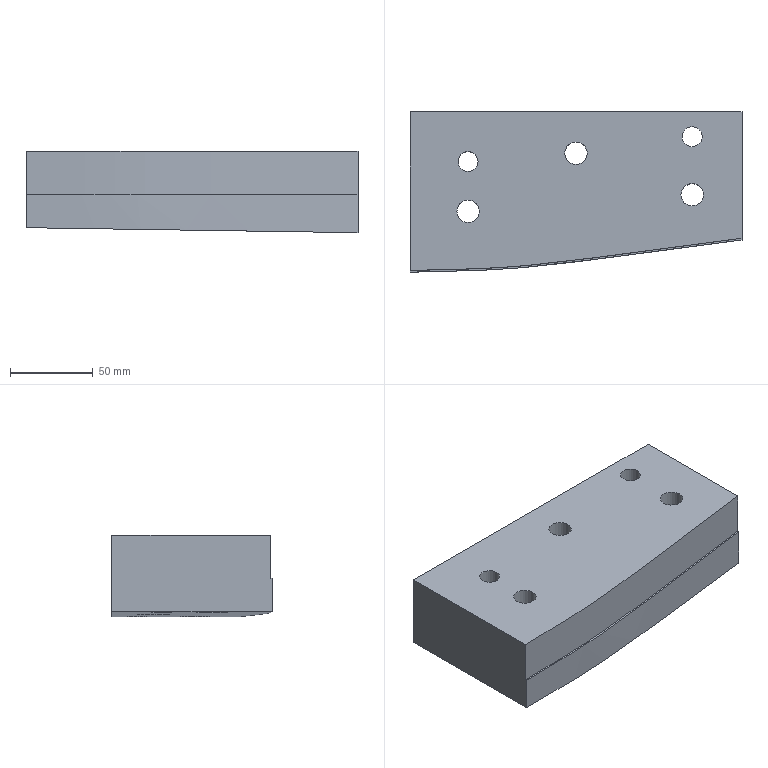Part | NX | features solid 2 | 1 solid | 23 faces | box 200 x 96.579 x 49 mm | volume 800737 mm3 | plane 11 | cylinder 10 | spline 2 | commonest cylinder face diameters 13.5 x3 19.5 x3 12 x2 13 x2
STEP:
#1=CARTESIAN_POINT('',(130.,110.798,14.));
#2=VERTEX_POINT('',#1);
#3=CARTESIAN_POINT('',(130.,111.807,14.));
#4=VERTEX_POINT('',#3);
#5=CARTESIAN_POINT('',(130.,154.403,14.));
#6=DIRECTION('',(0.,1.,0.));
#7=VECTOR('',#6,1000.);
#8=LINE('',#5,#7);
#9=EDGE_CURVE('',#2,#4,#8,.T.);
#10=ORIENTED_EDGE('',*,*,#9,.F.);
#11=CARTESIAN_POINT('',(130.,110.798,-9.));
#12=VERTEX_POINT('',#11);
#13=CARTESIAN_POINT('',(130.,110.798,15.5));
#14=DIRECTION('',(0.,0.,-1.));
#15=VECTOR('',#14,1000.);
#16=LINE('',#13,#15);
#17=EDGE_CURVE('',#12,#2,#16,.F.);
#18=ORIENTED_EDGE('',*,*,#17,.F.);
#19=CARTESIAN_POINT('',(130.,188.,-9.));
#20=VERTEX_POINT('',#19);
#21=CARTESIAN_POINT('',(130.,-222.,-9.));
#22=DIRECTION('',(0.,-1.,0.));
#23=VECTOR('',#22,1000.);
#24=LINE('',#21,#23);
#25=EDGE_CURVE('',#20,#12,#24,.T.);
#26=ORIENTED_EDGE('',*,*,#25,.F.);
#27=CARTESIAN_POINT('',(130.,188.,40.));
#28=VERTEX_POINT('',#27);
#29=CARTESIAN_POINT('',(130.,188.,-206.));
#30=DIRECTION('',(0.,0.,1.));
#31=VECTOR('',#30,1000.);
#32=LINE('',#29,#31);
#33=EDGE_CURVE('',#20,#28,#32,.T.);
#34=ORIENTED_EDGE('',*,*,#33,.T.);
#35=CARTESIAN_POINT('',(130.,111.807,40.));
#36=VERTEX_POINT('',#35);
#37=CARTESIAN_POINT('',(130.,35.09,40.));
#38=DIRECTION('',(0.,1.,0.));
#39=VECTOR('',#38,1000.);
#40=LINE('',#37,#39);
#41=EDGE_CURVE('',#36,#28,#40,.T.);
#42=ORIENTED_EDGE('',*,*,#41,.F.);
#43=CARTESIAN_POINT('',(130.,111.807,57.));
#44=DIRECTION('',(0.,0.,1.));
#45=VECTOR('',#44,1000.);
#46=LINE('',#43,#45);
#47=EDGE_CURVE('',#4,#36,#46,.T.);
#48=ORIENTED_EDGE('',*,*,#47,.F.);
#49=EDGE_LOOP('',(#10,#18,#26,#34,#42,#48));
#50=FACE_BOUND('',#49,.T.);
#51=CARTESIAN_POINT('',(130.,154.403,21.5));
#52=DIRECTION('',(1.,0.,0.));
#53=DIRECTION('',(0.,0.,-1.));
#54=AXIS2_PLACEMENT_3D('',#51,#52,#53);
#55=PLANE('',#54);
#56=ADVANCED_FACE('',(#50),#55,.T.);
#57=CARTESIAN_POINT('',(-70.,92.421,14.));
#58=VERTEX_POINT('',#57);
#59=CARTESIAN_POINT('',(-70.,91.421,14.));
#60=VERTEX_POINT('',#59);
#61=CARTESIAN_POINT('',(-70.,99.381,14.));
#62=DIRECTION('',(0.,-1.,0.));
#63=VECTOR('',#62,1000.);
#64=LINE('',#61,#63);
#65=EDGE_CURVE('',#58,#60,#64,.T.);
#66=ORIENTED_EDGE('',*,*,#65,.F.);
#67=CARTESIAN_POINT('',(-70.,92.421,40.));
#68=VERTEX_POINT('',#67);
#69=CARTESIAN_POINT('',(-70.,92.421,57.));
#70=DIRECTION('',(0.,0.,1.));
#71=VECTOR('',#70,1000.);
#72=LINE('',#69,#71);
#73=EDGE_CURVE('',#68,#58,#72,.F.);
#74=ORIENTED_EDGE('',*,*,#73,.F.);
#75=CARTESIAN_POINT('',(-70.,188.,40.));
#76=VERTEX_POINT('',#75);
#77=CARTESIAN_POINT('',(-70.,35.09,40.));
#78=DIRECTION('',(0.,-1.,0.));
#79=VECTOR('',#78,1000.);
#80=LINE('',#77,#79);
#81=EDGE_CURVE('',#76,#68,#80,.T.);
#82=ORIENTED_EDGE('',*,*,#81,.F.);
#83=CARTESIAN_POINT('',(-70.,188.,-6.));
#84=VERTEX_POINT('',#83);
#85=CARTESIAN_POINT('',(-70.,188.,-206.));
#86=DIRECTION('',(0.,0.,-1.));
#87=VECTOR('',#86,1000.);
#88=LINE('',#85,#87);
#89=EDGE_CURVE('',#76,#84,#88,.T.);
#90=ORIENTED_EDGE('',*,*,#89,.T.);
#91=CARTESIAN_POINT('',(-70.,91.421,-6.));
#92=VERTEX_POINT('',#91);
#93=CARTESIAN_POINT('',(-70.,-222.,-6.));
#94=DIRECTION('',(0.,1.,0.));
#95=VECTOR('',#94,1000.);
#96=LINE('',#93,#95);
#97=EDGE_CURVE('',#92,#84,#96,.T.);
#98=ORIENTED_EDGE('',*,*,#97,.F.);
#99=CARTESIAN_POINT('',(-70.,91.421,17.));
#100=DIRECTION('',(0.,0.,-1.));
#101=VECTOR('',#100,1000.);
#102=LINE('',#99,#101);
#103=EDGE_CURVE('',#92,#60,#102,.F.);
#104=ORIENTED_EDGE('',*,*,#103,.T.);
#105=EDGE_LOOP('',(#66,#74,#82,#90,#98,#104));
#106=FACE_BOUND('',#105,.T.);
#107=CARTESIAN_POINT('',(-70.,99.381,-66.));
#108=DIRECTION('',(-1.,0.,0.));
#109=DIRECTION('',(0.,0.,1.));
#110=AXIS2_PLACEMENT_3D('',#107,#108,#109);
#111=PLANE('',#110);
#112=ADVANCED_FACE('',(#106),#111,.T.);
#113=CARTESIAN_POINT('',(-190.231,-121.49,14.));
#114=CARTESIAN_POINT('',(-188.654,-121.152,14.));
#115=CARTESIAN_POINT('',(-185.47,-120.627,14.));
#116=CARTESIAN_POINT('',(-180.656,-120.141,14.));
#117=CARTESIAN_POINT('',(-175.882,-119.326,14.));
#118=CARTESIAN_POINT('',(-169.679,-117.528,14.));
#119=CARTESIAN_POINT('',(-162.185,-114.539,14.));
#120=CARTESIAN_POINT('',(-153.086,-111.254,14.));
#121=CARTESIAN_POINT('',(-144.031,-107.845,14.));
#122=CARTESIAN_POINT('',(-136.465,-105.061,14.));
#123=CARTESIAN_POINT('',(-130.418,-102.814,14.));
#124=CARTESIAN_POINT('',(-125.812,-101.329,14.));
#125=CARTESIAN_POINT('',(-121.306,-99.566,14.));
#126=CARTESIAN_POINT('',(-116.876,-97.626,14.));
#127=CARTESIAN_POINT('',(-112.335,-95.923,14.));
#128=CARTESIAN_POINT('',(-107.564,-95.05,14.));
#129=CARTESIAN_POINT('',(-102.756,-94.525,14.));
#130=CARTESIAN_POINT('',(-96.349,-93.771,14.));
#131=CARTESIAN_POINT('',(-89.902,-93.468,14.));
#132=CARTESIAN_POINT('',(-83.452,-93.448,14.));
#133=CARTESIAN_POINT('',(-77.002,-93.469,14.));
#134=CARTESIAN_POINT('',(-68.939,-93.411,14.));
#135=CARTESIAN_POINT('',(-56.04,-93.3,14.));
#136=CARTESIAN_POINT('',(-33.465,-93.184,14.));
#137=CARTESIAN_POINT('',(-7.666,-93.074,14.));
#138=CARTESIAN_POINT('',(14.907,-92.653,14.));
#139=CARTESIAN_POINT('',(27.794,-92.068,14.));
#140=CARTESIAN_POINT('',(40.668,-91.245,14.));
#141=CARTESIAN_POINT('',(51.917,-90.291,14.));
#142=CARTESIAN_POINT('',(61.528,-89.174,14.));
#143=CARTESIAN_POINT('',(67.939,-88.466,14.));
#144=CARTESIAN_POINT('',(79.125,-86.95,14.));
#145=CARTESIAN_POINT('',(95.161,-85.253,14.));
#146=CARTESIAN_POINT('',(114.404,-83.21,14.));
#147=CARTESIAN_POINT('',(133.568,-80.524,14.));
#148=CARTESIAN_POINT('',(152.734,-77.861,14.));
#149=CARTESIAN_POINT('',(171.916,-75.326,14.));
#150=CARTESIAN_POINT('',(191.055,-72.413,14.));
#151=CARTESIAN_POINT('',(207.17,-71.468,14.));
#152=CARTESIAN_POINT('',(219.951,-69.697,14.));
#153=CARTESIAN_POINT('',(232.724,-67.899,14.));
#154=CARTESIAN_POINT('',(248.708,-65.766,14.));
#155=CARTESIAN_POINT('',(267.87,-63.074,14.));
#156=CARTESIAN_POINT('',(287.038,-60.44,14.));
#157=CARTESIAN_POINT('',(301.448,-58.682,14.));
#158=CARTESIAN_POINT('',(310.976,-56.987,14.));
#159=CARTESIAN_POINT('',(314.916,-56.135,14.));
#160=CARTESIAN_POINT('',(318.052,-55.382,14.));
#161=CARTESIAN_POINT('',(320.39,-54.76,14.));
#162=CARTESIAN_POINT('',(322.686,-53.981,14.));
#163=CARTESIAN_POINT('',(325.595,-52.578,14.));
#164=CARTESIAN_POINT('',(328.769,-50.098,14.));
#165=CARTESIAN_POINT('',(332.247,-46.69,14.));
#166=CARTESIAN_POINT('',(335.795,-43.406,14.));
#167=CARTESIAN_POINT('',(343.661,-37.758,14.));
#168=CARTESIAN_POINT('',(355.164,-28.914,14.));
#169=CARTESIAN_POINT('',(370.422,-17.018,14.));
#170=CARTESIAN_POINT('',(383.264,-7.249,14.));
#171=CARTESIAN_POINT('',(392.416,-0.6713,14.));
#172=CARTESIAN_POINT('',(396.953,2.733,14.));
#173=CARTESIAN_POINT('',(398.886,5.372,14.));
#174=CARTESIAN_POINT('',(399.725,7.654,14.));
#175=CARTESIAN_POINT('',(399.76,10.078,14.));
#176=CARTESIAN_POINT('',(399.483,13.317,14.));
#177=CARTESIAN_POINT('',(399.712,17.34,14.));
#178=CARTESIAN_POINT('',(399.612,22.179,14.));
#179=CARTESIAN_POINT('',(399.633,31.854,14.));
#180=CARTESIAN_POINT('',(399.593,46.366,14.));
#181=CARTESIAN_POINT('',(399.637,62.491,14.));
#182=CARTESIAN_POINT('',(399.588,73.779,14.));
#183=CARTESIAN_POINT('',(399.652,79.422,14.));
#184=CARTESIAN_POINT('',(399.59,82.647,14.));
#185=CARTESIAN_POINT('',(399.564,85.065,14.));
#186=CARTESIAN_POINT('',(399.725,87.486,14.));
#187=CARTESIAN_POINT('',(399.756,89.902,14.));
#188=CARTESIAN_POINT('',(399.247,92.301,14.));
#189=CARTESIAN_POINT('',(397.362,95.008,14.));
#190=CARTESIAN_POINT('',(393.635,96.774,14.));
#191=CARTESIAN_POINT('',(389.279,98.826,14.));
#192=CARTESIAN_POINT('',(384.732,100.498,14.));
#193=CARTESIAN_POINT('',(378.765,102.95,14.));
#194=CARTESIAN_POINT('',(362.589,110.229,14.));
#195=CARTESIAN_POINT('',(344.928,118.135,14.));
#196=CARTESIAN_POINT('',(327.281,126.072,14.));
#197=CARTESIAN_POINT('',(319.932,129.381,14.));
#198=CARTESIAN_POINT('',(314.075,132.102,14.));
#199=CARTESIAN_POINT('',(309.387,133.376,14.));
#200=CARTESIAN_POINT('',(304.547,133.785,14.));
#201=CARTESIAN_POINT('',(299.716,133.401,14.));
#202=CARTESIAN_POINT('',(294.929,132.704,14.));
#203=CARTESIAN_POINT('',(288.543,131.8,14.));
#204=CARTESIAN_POINT('',(277.364,130.241,14.));
#205=CARTESIAN_POINT('',(242.2,125.552,14.));
#206=CARTESIAN_POINT('',(184.637,118.048,14.));
#207=CARTESIAN_POINT('',(120.701,109.541,14.));
#208=CARTESIAN_POINT('',(69.531,102.902,14.));
#209=CARTESIAN_POINT('',(40.777,98.94,14.));
#210=CARTESIAN_POINT('',(21.566,96.615,14.));
#211=CARTESIAN_POINT('',(8.743,95.212,14.));
#212=CARTESIAN_POINT('',(-7.301,93.575,14.));
#213=CARTESIAN_POINT('',(-26.625,92.505,14.));
#214=CARTESIAN_POINT('',(-45.971,92.017,14.));
#215=CARTESIAN_POINT('',(-62.09,91.675,14.));
#216=CARTESIAN_POINT('',(-74.987,91.256,14.));
#217=CARTESIAN_POINT('',(-84.664,91.165,14.));
#218=CARTESIAN_POINT('',(-94.319,91.781,14.));
#219=CARTESIAN_POINT('',(-103.929,92.966,14.));
#220=CARTESIAN_POINT('',(-113.495,94.403,14.));
#221=CARTESIAN_POINT('',(-119.856,95.492,14.));
#222=CARTESIAN_POINT('',(-122.997,96.222,14.));
#223=B_SPLINE_CURVE_WITH_KNOTS('',3,(#113,#114,#115,#116,#117,#118,#119,#120,#121,#122,#123,#124,#125,#126,#127,#128,#129,#130,#131,#132,#133,#134,#135,#136,#137,#138,#139,#140,#141,#142,#143,#144,#145,#146,#147,#148,#149,#150,#151,#152,#153,#154,#155,#156,#157,#158,#159,#160,#161,#162,#163,#164,#165,#166,#167,#168,#169,#170,#171,#172,#173,#174,#175,#176,#177,#178,#179,#180,#181,#182,#183,#184,#185,#186,#187,#188,#189,#190,#191,#192,#193,#194,#195,#196,#197,#198,#199,#200,#201,#202,#203,#204,#205,#206,#207,#208,#209,#210,#211,#212,#213,#214,#215,#216,#217,#218,#219,#220,#221,#222),.UNSPECIFIED.,.F.,.F.,(4,1,1,1,1,1,1,1,1,1,1,1,1,1,1,1,1,1,1,1,1,1,1,1,1,1,1,1,1,1,1,1,1,1,1,1,1,1,1,1,1,1,1,1,1,1,1,1,1,1,1,1,1,1,1,1,1,1,1,1,1,1,1,1,1,1,1,1,1,1,1,1,1,1,1,1,1,1,1,1,1,1,1,1,1,1,1,1,1,1,1,1,1,1,1,1,1,1,1,1,1,1,1,1,1,1,1,4),(0.4704,0.4724,0.4745,0.4766,0.4786,0.4828,0.4869,0.491,0.4952,0.4972,0.4993,0.5014,0.5035,0.5055,0.5076,0.5097,0.5117,0.5159,0.5179,0.52,0.5241,0.5283,0.5366,0.5531,0.5614,0.5655,0.5697,0.5779,0.58,0.5821,0.5862,0.5945,0.6028,0.611,0.6193,0.6276,0.6359,0.6441,0.6483,0.6524,0.6607,0.669,0.6772,0.6855,0.6876,0.6897,0.6907,0.6917,0.6928,0.6938,0.6959,0.6979,0.7,0.7021,0.7103,0.7186,0.7269,0.731,0.7331,0.7341,0.7352,0.7362,0.7372,0.7393,0.7414,0.7435,0.7517,0.76,0.7641,0.7662,0.7672,0.7683,0.7693,0.7703,0.7714,0.7724,0.7745,0.7766,0.7786,0.7807,0.7848,0.8014,0.8055,0.8097,0.8117,0.8138,0.8159,0.8179,0.82,0.8221,0.8262,0.8345,0.8676,0.9007,0.9172,0.9338,0.9379,0.9421,0.9503,0.9586,0.9669,0.9752,0.9793,0.9834,0.9876,0.9917,0.9959,1.),.UNSPECIFIED.);
#224=EDGE_CURVE('',#60,#2,#223,.F.);
#225=ORIENTED_EDGE('',*,*,#224,.F.);
#226=ORIENTED_EDGE('',*,*,#103,.F.);
#227=CARTESIAN_POINT('',(-70.,91.421,-6.));
#228=CARTESIAN_POINT('',(-61.612,91.662,-6.126));
#229=CARTESIAN_POINT('',(-44.826,92.047,-6.378));
#230=CARTESIAN_POINT('',(-19.653,92.685,-6.755));
#231=CARTESIAN_POINT('',(5.381,94.749,-7.131));
#232=CARTESIAN_POINT('',(38.657,98.573,-7.63));
#233=CARTESIAN_POINT('',(80.155,104.356,-8.252));
#234=CARTESIAN_POINT('',(113.389,108.608,-8.751));
#235=CARTESIAN_POINT('',(130.,110.798,-9.));
#236=B_SPLINE_CURVE_WITH_KNOTS('',3,(#227,#228,#229,#230,#231,#232,#233,#234,#235),.UNSPECIFIED.,.F.,.F.,(4,1,1,1,1,1,4),(0.,0.02512,0.05024,0.07536,0.1005,0.1507,0.201),.UNSPECIFIED.);
#237=EDGE_CURVE('',#92,#12,#236,.T.);
#238=ORIENTED_EDGE('',*,*,#237,.T.);
#239=ORIENTED_EDGE('',*,*,#17,.T.);
#240=EDGE_LOOP('',(#225,#226,#238,#239));
#241=FACE_BOUND('',#240,.T.);
#242=CARTESIAN_POINT('',(130.,110.798,14.));
#243=CARTESIAN_POINT('',(130.,110.798,-9.138));
#244=CARTESIAN_POINT('',(113.384,108.607,14.));
#245=CARTESIAN_POINT('',(113.384,108.607,-9.138));
#246=CARTESIAN_POINT('',(88.451,105.393,14.));
#247=CARTESIAN_POINT('',(88.451,105.393,-9.138));
#248=CARTESIAN_POINT('',(55.23,100.923,14.));
#249=CARTESIAN_POINT('',(55.23,100.923,-9.138));
#250=CARTESIAN_POINT('',(30.311,97.595,14.));
#251=CARTESIAN_POINT('',(30.311,97.595,-9.138));
#252=CARTESIAN_POINT('',(9.491,95.247,14.));
#253=CARTESIAN_POINT('',(9.491,95.247,-9.138));
#254=CARTESIAN_POINT('',(-7.195,93.67,14.));
#255=CARTESIAN_POINT('',(-7.195,93.67,-9.138));
#256=CARTESIAN_POINT('',(-23.922,92.6,14.));
#257=CARTESIAN_POINT('',(-23.922,92.6,-9.138));
#258=CARTESIAN_POINT('',(-44.868,92.037,14.));
#259=CARTESIAN_POINT('',(-44.868,92.037,-9.138));
#260=CARTESIAN_POINT('',(-61.621,91.662,14.));
#261=CARTESIAN_POINT('',(-61.621,91.662,-9.138));
#262=CARTESIAN_POINT('',(-70.,91.421,14.));
#263=CARTESIAN_POINT('',(-70.,91.421,-9.138));
#264=B_SPLINE_SURFACE_WITH_KNOTS('',3,1,((#242,#243),(#244,#245),(#246,#247),(#248,#249),(#250,#251),(#252,#253),(#254,#255),(#256,#257),(#258,#259),(#260,#261),(#262,#263)),.SURF_OF_LINEAR_EXTRUSION.,.F.,.F.,.F.,(4,1,1,1,1,1,1,1,4),(2,2),(0.8912,0.9127,0.9234,0.9342,0.9449,0.9503,0.9557,0.9664,0.9772),(0.,1.),.UNSPECIFIED.);
#265=ADVANCED_FACE('',(#241),#264,.T.);
#266=ORIENTED_EDGE('',*,*,#33,.F.);
#267=CARTESIAN_POINT('',(-470.284,188.,0.004265));
#268=DIRECTION('',(0.9999,0.,-0.015));
#269=VECTOR('',#268,1000.);
#270=LINE('',#267,#269);
#271=EDGE_CURVE('',#84,#20,#270,.T.);
#272=ORIENTED_EDGE('',*,*,#271,.F.);
#273=ORIENTED_EDGE('',*,*,#89,.F.);
#274=CARTESIAN_POINT('',(-415.478,188.,40.));
#275=DIRECTION('',(1.,0.,0.));
#276=VECTOR('',#275,1000.);
#277=LINE('',#274,#276);
#278=EDGE_CURVE('',#76,#28,#277,.T.);
#279=ORIENTED_EDGE('',*,*,#278,.T.);
#280=EDGE_LOOP('',(#266,#272,#273,#279));
#281=FACE_BOUND('',#280,.T.);
#282=CARTESIAN_POINT('',(-470.374,188.,-206.));
#283=DIRECTION('',(0.,-1.,0.));
#284=DIRECTION('',(1.,0.,0.));
#285=AXIS2_PLACEMENT_3D('',#282,#283,#284);
#286=PLANE('',#285);
#287=ADVANCED_FACE('',(#281),#286,.F.);
#288=CARTESIAN_POINT('',(130.,111.807,40.));
#289=CARTESIAN_POINT('',(113.389,109.617,40.));
#290=CARTESIAN_POINT('',(80.155,105.364,40.));
#291=CARTESIAN_POINT('',(38.657,99.582,40.));
#292=CARTESIAN_POINT('',(5.382,95.754,40.));
#293=CARTESIAN_POINT('',(-19.653,93.685,40.));
#294=CARTESIAN_POINT('',(-44.826,93.047,40.));
#295=CARTESIAN_POINT('',(-61.612,92.663,40.));
#296=CARTESIAN_POINT('',(-70.,92.421,40.));
#297=B_SPLINE_CURVE_WITH_KNOTS('',3,(#288,#289,#290,#291,#292,#293,#294,#295,#296),.UNSPECIFIED.,.F.,.F.,(4,1,1,1,1,1,4),(0.,0.05023,0.1005,0.1256,0.1507,0.1758,0.2009),.UNSPECIFIED.);
#298=EDGE_CURVE('',#36,#68,#297,.T.);
#299=ORIENTED_EDGE('',*,*,#298,.F.);
#300=ORIENTED_EDGE('',*,*,#41,.T.);
#301=ORIENTED_EDGE('',*,*,#278,.F.);
#302=ORIENTED_EDGE('',*,*,#81,.T.);
#303=EDGE_LOOP('',(#299,#300,#301,#302));
#304=FACE_BOUND('',#303,.T.);
#305=CARTESIAN_POINT('',(106.,173.,40.));
#306=VERTEX_POINT('',#305);
#307=CARTESIAN_POINT('',(100.,173.,40.));
#308=DIRECTION('',(0.,0.,1.));
#309=DIRECTION('',(1.,0.,0.));
#310=AXIS2_PLACEMENT_3D('',#307,#308,#309);
#311=CIRCLE('',#310,6.);
#312=EDGE_CURVE('',#306,#306,#311,.T.);
#313=ORIENTED_EDGE('',*,*,#312,.F.);
#314=EDGE_LOOP('',(#313));
#315=FACE_BOUND('',#314,.T.);
#316=CARTESIAN_POINT('',(-29.,158.,40.));
#317=VERTEX_POINT('',#316);
#318=CARTESIAN_POINT('',(-35.,158.,40.));
#319=DIRECTION('',(0.,0.,1.));
#320=DIRECTION('',(1.,0.,0.));
#321=AXIS2_PLACEMENT_3D('',#318,#319,#320);
#322=CIRCLE('',#321,6.);
#323=EDGE_CURVE('',#317,#317,#322,.T.);
#324=ORIENTED_EDGE('',*,*,#323,.F.);
#325=EDGE_LOOP('',(#324));
#326=FACE_BOUND('',#325,.T.);
#327=CARTESIAN_POINT('',(36.75,163.,40.));
#328=VERTEX_POINT('',#327);
#329=CARTESIAN_POINT('',(30.,163.,40.));
#330=DIRECTION('',(0.,0.,1.));
#331=DIRECTION('',(1.,0.,0.));
#332=AXIS2_PLACEMENT_3D('',#329,#330,#331);
#333=CIRCLE('',#332,6.75);
#334=EDGE_CURVE('',#328,#328,#333,.T.);
#335=ORIENTED_EDGE('',*,*,#334,.F.);
#336=EDGE_LOOP('',(#335));
#337=FACE_BOUND('',#336,.T.);
#338=CARTESIAN_POINT('',(-28.25,128.,40.));
#339=VERTEX_POINT('',#338);
#340=CARTESIAN_POINT('',(-35.,128.,40.));
#341=DIRECTION('',(0.,0.,1.));
#342=DIRECTION('',(1.,0.,0.));
#343=AXIS2_PLACEMENT_3D('',#340,#341,#342);
#344=CIRCLE('',#343,6.75);
#345=EDGE_CURVE('',#339,#339,#344,.T.);
#346=ORIENTED_EDGE('',*,*,#345,.F.);
#347=EDGE_LOOP('',(#346));
#348=FACE_BOUND('',#347,.T.);
#349=CARTESIAN_POINT('',(106.75,138.,40.));
#350=VERTEX_POINT('',#349);
#351=CARTESIAN_POINT('',(100.,138.,40.));
#352=DIRECTION('',(0.,0.,1.));
#353=DIRECTION('',(1.,0.,0.));
#354=AXIS2_PLACEMENT_3D('',#351,#352,#353);
#355=CIRCLE('',#354,6.75);
#356=EDGE_CURVE('',#350,#350,#355,.T.);
#357=ORIENTED_EDGE('',*,*,#356,.F.);
#358=EDGE_LOOP('',(#357));
#359=FACE_BOUND('',#358,.T.);
#360=CARTESIAN_POINT('',(-415.478,35.09,40.));
#361=DIRECTION('',(0.,0.,1.));
#362=DIRECTION('',(1.,0.,0.));
#363=AXIS2_PLACEMENT_3D('',#360,#361,#362);
#364=PLANE('',#363);
#365=ADVANCED_FACE('',(#304,#315,#326,#337,#348,#359),#364,.T.);
#366=ORIENTED_EDGE('',*,*,#356,.T.);
#367=EDGE_LOOP('',(#366));
#368=FACE_BOUND('',#367,.T.);
#369=CARTESIAN_POINT('',(106.75,138.,9.));
#370=VERTEX_POINT('',#369);
#371=CARTESIAN_POINT('',(100.,138.,9.));
#372=DIRECTION('',(0.,0.,1.));
#373=DIRECTION('',(1.,0.,0.));
#374=AXIS2_PLACEMENT_3D('',#371,#372,#373);
#375=CIRCLE('',#374,6.75);
#376=EDGE_CURVE('',#370,#370,#375,.T.);
#377=ORIENTED_EDGE('',*,*,#376,.F.);
#378=EDGE_LOOP('',(#377));
#379=FACE_BOUND('',#378,.T.);
#380=CARTESIAN_POINT('',(100.,138.,94.));
#381=DIRECTION('',(0.,0.,1.));
#382=DIRECTION('',(1.,0.,0.));
#383=AXIS2_PLACEMENT_3D('',#380,#381,#382);
#384=CYLINDRICAL_SURFACE('',#383,6.75);
#385=ADVANCED_FACE('',(#368,#379),#384,.F.);
#386=ORIENTED_EDGE('',*,*,#376,.T.);
#387=EDGE_LOOP('',(#386));
#388=FACE_BOUND('',#387,.T.);
#389=CARTESIAN_POINT('',(109.75,138.,9.));
#390=VERTEX_POINT('',#389);
#391=CARTESIAN_POINT('',(100.,138.,9.));
#392=DIRECTION('',(0.,0.,1.));
#393=DIRECTION('',(1.,0.,0.));
#394=AXIS2_PLACEMENT_3D('',#391,#392,#393);
#395=CIRCLE('',#394,9.75);
#396=EDGE_CURVE('',#390,#390,#395,.T.);
#397=ORIENTED_EDGE('',*,*,#396,.F.);
#398=EDGE_LOOP('',(#397));
#399=FACE_BOUND('',#398,.T.);
#400=CARTESIAN_POINT('',(100.,138.,9.));
#401=DIRECTION('',(0.,0.,1.));
#402=DIRECTION('',(1.,0.,0.));
#403=AXIS2_PLACEMENT_3D('',#400,#401,#402);
#404=PLANE('',#403);
#405=ADVANCED_FACE('',(#388,#399),#404,.F.);
#406=ORIENTED_EDGE('',*,*,#396,.T.);
#407=EDGE_LOOP('',(#406));
#408=FACE_BOUND('',#407,.T.);
#409=CARTESIAN_POINT('',(109.75,138.,-8.696));
#410=VERTEX_POINT('',#409);
#411=CARTESIAN_POINT('',(100.,138.,-8.55));
#412=DIRECTION('',(0.015,0.,0.9999));
#413=DIRECTION('',(0.9999,0.,-0.015));
#414=AXIS2_PLACEMENT_3D('',#411,#412,#413);
#415=ELLIPSE('',#414,9.751,9.75);
#416=EDGE_CURVE('',#410,#410,#415,.T.);
#417=ORIENTED_EDGE('',*,*,#416,.F.);
#418=EDGE_LOOP('',(#417));
#419=FACE_BOUND('',#418,.T.);
#420=CARTESIAN_POINT('',(100.,138.,-6.));
#421=DIRECTION('',(0.,0.,1.));
#422=DIRECTION('',(1.,0.,0.));
#423=AXIS2_PLACEMENT_3D('',#420,#421,#422);
#424=CYLINDRICAL_SURFACE('',#423,9.75);
#425=ADVANCED_FACE('',(#408,#419),#424,.F.);
#426=ORIENTED_EDGE('',*,*,#345,.T.);
#427=EDGE_LOOP('',(#426));
#428=FACE_BOUND('',#427,.T.);
#429=CARTESIAN_POINT('',(-28.25,128.,9.));
#430=VERTEX_POINT('',#429);
#431=CARTESIAN_POINT('',(-35.,128.,9.));
#432=DIRECTION('',(0.,0.,1.));
#433=DIRECTION('',(1.,0.,0.));
#434=AXIS2_PLACEMENT_3D('',#431,#432,#433);
#435=CIRCLE('',#434,6.75);
#436=EDGE_CURVE('',#430,#430,#435,.T.);
#437=ORIENTED_EDGE('',*,*,#436,.F.);
#438=EDGE_LOOP('',(#437));
#439=FACE_BOUND('',#438,.T.);
#440=CARTESIAN_POINT('',(-35.,128.,94.));
#441=DIRECTION('',(0.,0.,1.));
#442=DIRECTION('',(1.,0.,0.));
#443=AXIS2_PLACEMENT_3D('',#440,#441,#442);
#444=CYLINDRICAL_SURFACE('',#443,6.75);
#445=ADVANCED_FACE('',(#428,#439),#444,.F.);
#446=ORIENTED_EDGE('',*,*,#436,.T.);
#447=EDGE_LOOP('',(#446));
#448=FACE_BOUND('',#447,.T.);
#449=CARTESIAN_POINT('',(-25.25,128.,9.));
#450=VERTEX_POINT('',#449);
#451=CARTESIAN_POINT('',(-35.,128.,9.));
#452=DIRECTION('',(0.,0.,1.));
#453=DIRECTION('',(1.,0.,0.));
#454=AXIS2_PLACEMENT_3D('',#451,#452,#453);
#455=CIRCLE('',#454,9.75);
#456=EDGE_CURVE('',#450,#450,#455,.T.);
#457=ORIENTED_EDGE('',*,*,#456,.F.);
#458=EDGE_LOOP('',(#457));
#459=FACE_BOUND('',#458,.T.);
#460=CARTESIAN_POINT('',(-35.,128.,9.));
#461=DIRECTION('',(0.,0.,1.));
#462=DIRECTION('',(1.,0.,0.));
#463=AXIS2_PLACEMENT_3D('',#460,#461,#462);
#464=PLANE('',#463);
#465=ADVANCED_FACE('',(#448,#459),#464,.F.);
#466=ORIENTED_EDGE('',*,*,#456,.T.);
#467=EDGE_LOOP('',(#466));
#468=FACE_BOUND('',#467,.T.);
#469=CARTESIAN_POINT('',(-25.25,128.,-6.671));
#470=VERTEX_POINT('',#469);
#471=CARTESIAN_POINT('',(-35.,128.,-6.525));
#472=DIRECTION('',(0.015,0.,0.9999));
#473=DIRECTION('',(0.9999,0.,-0.015));
#474=AXIS2_PLACEMENT_3D('',#471,#472,#473);
#475=ELLIPSE('',#474,9.751,9.75);
#476=EDGE_CURVE('',#470,#470,#475,.T.);
#477=ORIENTED_EDGE('',*,*,#476,.F.);
#478=EDGE_LOOP('',(#477));
#479=FACE_BOUND('',#478,.T.);
#480=CARTESIAN_POINT('',(-35.,128.,-6.));
#481=DIRECTION('',(0.,0.,1.));
#482=DIRECTION('',(1.,0.,0.));
#483=AXIS2_PLACEMENT_3D('',#480,#481,#482);
#484=CYLINDRICAL_SURFACE('',#483,9.75);
#485=ADVANCED_FACE('',(#468,#479),#484,.F.);
#486=ORIENTED_EDGE('',*,*,#334,.T.);
#487=EDGE_LOOP('',(#486));
#488=FACE_BOUND('',#487,.T.);
#489=CARTESIAN_POINT('',(36.75,163.,9.));
#490=VERTEX_POINT('',#489);
#491=CARTESIAN_POINT('',(30.,163.,9.));
#492=DIRECTION('',(0.,0.,1.));
#493=DIRECTION('',(1.,0.,0.));
#494=AXIS2_PLACEMENT_3D('',#491,#492,#493);
#495=CIRCLE('',#494,6.75);
#496=EDGE_CURVE('',#490,#490,#495,.T.);
#497=ORIENTED_EDGE('',*,*,#496,.F.);
#498=EDGE_LOOP('',(#497));
#499=FACE_BOUND('',#498,.T.);
#500=CARTESIAN_POINT('',(30.,163.,94.));
#501=DIRECTION('',(0.,0.,1.));
#502=DIRECTION('',(1.,0.,0.));
#503=AXIS2_PLACEMENT_3D('',#500,#501,#502);
#504=CYLINDRICAL_SURFACE('',#503,6.75);
#505=ADVANCED_FACE('',(#488,#499),#504,.F.);
#506=ORIENTED_EDGE('',*,*,#496,.T.);
#507=EDGE_LOOP('',(#506));
#508=FACE_BOUND('',#507,.T.);
#509=CARTESIAN_POINT('',(39.75,163.,9.));
#510=VERTEX_POINT('',#509);
#511=CARTESIAN_POINT('',(30.,163.,9.));
#512=DIRECTION('',(0.,0.,1.));
#513=DIRECTION('',(1.,0.,0.));
#514=AXIS2_PLACEMENT_3D('',#511,#512,#513);
#515=CIRCLE('',#514,9.75);
#516=EDGE_CURVE('',#510,#510,#515,.T.);
#517=ORIENTED_EDGE('',*,*,#516,.F.);
#518=EDGE_LOOP('',(#517));
#519=FACE_BOUND('',#518,.T.);
#520=CARTESIAN_POINT('',(30.,163.,9.));
#521=DIRECTION('',(0.,0.,1.));
#522=DIRECTION('',(1.,0.,0.));
#523=AXIS2_PLACEMENT_3D('',#520,#521,#522);
#524=PLANE('',#523);
#525=ADVANCED_FACE('',(#508,#519),#524,.F.);
#526=ORIENTED_EDGE('',*,*,#516,.T.);
#527=EDGE_LOOP('',(#526));
#528=FACE_BOUND('',#527,.T.);
#529=CARTESIAN_POINT('',(39.75,163.,-7.646));
#530=VERTEX_POINT('',#529);
#531=CARTESIAN_POINT('',(30.,163.,-7.5));
#532=DIRECTION('',(0.015,0.,0.9999));
#533=DIRECTION('',(0.9999,0.,-0.015));
#534=AXIS2_PLACEMENT_3D('',#531,#532,#533);
#535=ELLIPSE('',#534,9.751,9.75);
#536=EDGE_CURVE('',#530,#530,#535,.T.);
#537=ORIENTED_EDGE('',*,*,#536,.F.);
#538=EDGE_LOOP('',(#537));
#539=FACE_BOUND('',#538,.T.);
#540=CARTESIAN_POINT('',(30.,163.,-6.));
#541=DIRECTION('',(0.,0.,1.));
#542=DIRECTION('',(1.,0.,0.));
#543=AXIS2_PLACEMENT_3D('',#540,#541,#542);
#544=CYLINDRICAL_SURFACE('',#543,9.75);
#545=ADVANCED_FACE('',(#528,#539),#544,.F.);
#546=ORIENTED_EDGE('',*,*,#323,.T.);
#547=EDGE_LOOP('',(#546));
#548=FACE_BOUND('',#547,.T.);
#549=CARTESIAN_POINT('',(-29.,158.,14.));
#550=VERTEX_POINT('',#549);
#551=CARTESIAN_POINT('',(-35.,158.,14.));
#552=DIRECTION('',(0.,0.,1.));
#553=DIRECTION('',(1.,0.,0.));
#554=AXIS2_PLACEMENT_3D('',#551,#552,#553);
#555=CIRCLE('',#554,6.);
#556=EDGE_CURVE('',#550,#550,#555,.T.);
#557=ORIENTED_EDGE('',*,*,#556,.F.);
#558=EDGE_LOOP('',(#557));
#559=FACE_BOUND('',#558,.T.);
#560=CARTESIAN_POINT('',(-35.,158.,94.));
#561=DIRECTION('',(0.,0.,1.));
#562=DIRECTION('',(1.,0.,0.));
#563=AXIS2_PLACEMENT_3D('',#560,#561,#562);
#564=CYLINDRICAL_SURFACE('',#563,6.);
#565=ADVANCED_FACE('',(#548,#559),#564,.F.);
#566=ORIENTED_EDGE('',*,*,#556,.T.);
#567=EDGE_LOOP('',(#566));
#568=FACE_BOUND('',#567,.T.);
#569=CARTESIAN_POINT('',(-28.5,158.,14.));
#570=VERTEX_POINT('',#569);
#571=CARTESIAN_POINT('',(-35.,158.,14.));
#572=DIRECTION('',(0.,0.,1.));
#573=DIRECTION('',(1.,0.,0.));
#574=AXIS2_PLACEMENT_3D('',#571,#572,#573);
#575=CIRCLE('',#574,6.5);
#576=EDGE_CURVE('',#570,#570,#575,.T.);
#577=ORIENTED_EDGE('',*,*,#576,.F.);
#578=EDGE_LOOP('',(#577));
#579=FACE_BOUND('',#578,.T.);
#580=CARTESIAN_POINT('',(-35.,163.,14.));
#581=DIRECTION('',(0.,0.,1.));
#582=DIRECTION('',(1.,0.,0.));
#583=AXIS2_PLACEMENT_3D('',#580,#581,#582);
#584=PLANE('',#583);
#585=ADVANCED_FACE('',(#568,#579),#584,.F.);
#586=ORIENTED_EDGE('',*,*,#576,.T.);
#587=EDGE_LOOP('',(#586));
#588=FACE_BOUND('',#587,.T.);
#589=CARTESIAN_POINT('',(-28.5,158.,-6.622));
#590=VERTEX_POINT('',#589);
#591=CARTESIAN_POINT('',(-35.,158.,-6.525));
#592=DIRECTION('',(0.015,0.,0.9999));
#593=DIRECTION('',(0.9999,0.,-0.015));
#594=AXIS2_PLACEMENT_3D('',#591,#592,#593);
#595=ELLIPSE('',#594,6.501,6.5);
#596=EDGE_CURVE('',#590,#590,#595,.T.);
#597=ORIENTED_EDGE('',*,*,#596,.F.);
#598=EDGE_LOOP('',(#597));
#599=FACE_BOUND('',#598,.T.);
#600=CARTESIAN_POINT('',(-35.,158.,-6.));
#601=DIRECTION('',(0.,0.,1.));
#602=DIRECTION('',(1.,0.,0.));
#603=AXIS2_PLACEMENT_3D('',#600,#601,#602);
#604=CYLINDRICAL_SURFACE('',#603,6.5);
#605=ADVANCED_FACE('',(#588,#599),#604,.F.);
#606=ORIENTED_EDGE('',*,*,#312,.T.);
#607=EDGE_LOOP('',(#606));
#608=FACE_BOUND('',#607,.T.);
#609=CARTESIAN_POINT('',(106.,173.,14.));
#610=VERTEX_POINT('',#609);
#611=CARTESIAN_POINT('',(100.,173.,14.));
#612=DIRECTION('',(0.,0.,1.));
#613=DIRECTION('',(1.,0.,0.));
#614=AXIS2_PLACEMENT_3D('',#611,#612,#613);
#615=CIRCLE('',#614,6.);
#616=EDGE_CURVE('',#610,#610,#615,.T.);
#617=ORIENTED_EDGE('',*,*,#616,.F.);
#618=EDGE_LOOP('',(#617));
#619=FACE_BOUND('',#618,.T.);
#620=CARTESIAN_POINT('',(100.,173.,94.));
#621=DIRECTION('',(0.,0.,1.));
#622=DIRECTION('',(1.,0.,0.));
#623=AXIS2_PLACEMENT_3D('',#620,#621,#622);
#624=CYLINDRICAL_SURFACE('',#623,6.);
#625=ADVANCED_FACE('',(#608,#619),#624,.F.);
#626=ORIENTED_EDGE('',*,*,#616,.T.);
#627=EDGE_LOOP('',(#626));
#628=FACE_BOUND('',#627,.T.);
#629=CARTESIAN_POINT('',(106.5,173.,14.));
#630=VERTEX_POINT('',#629);
#631=CARTESIAN_POINT('',(100.,173.,14.));
#632=DIRECTION('',(0.,0.,1.));
#633=DIRECTION('',(1.,0.,0.));
#634=AXIS2_PLACEMENT_3D('',#631,#632,#633);
#635=CIRCLE('',#634,6.5);
#636=EDGE_CURVE('',#630,#630,#635,.T.);
#637=ORIENTED_EDGE('',*,*,#636,.F.);
#638=EDGE_LOOP('',(#637));
#639=FACE_BOUND('',#638,.T.);
#640=CARTESIAN_POINT('',(100.,173.,14.));
#641=DIRECTION('',(0.,0.,1.));
#642=DIRECTION('',(1.,0.,0.));
#643=AXIS2_PLACEMENT_3D('',#640,#641,#642);
#644=PLANE('',#643);
#645=ADVANCED_FACE('',(#628,#639),#644,.F.);
#646=ORIENTED_EDGE('',*,*,#636,.T.);
#647=EDGE_LOOP('',(#646));
#648=FACE_BOUND('',#647,.T.);
#649=CARTESIAN_POINT('',(106.5,173.,-8.648));
#650=VERTEX_POINT('',#649);
#651=CARTESIAN_POINT('',(100.,173.,-8.55));
#652=DIRECTION('',(0.015,0.,0.9999));
#653=DIRECTION('',(0.9999,0.,-0.015));
#654=AXIS2_PLACEMENT_3D('',#651,#652,#653);
#655=ELLIPSE('',#654,6.501,6.5);
#656=EDGE_CURVE('',#650,#650,#655,.T.);
#657=ORIENTED_EDGE('',*,*,#656,.F.);
#658=EDGE_LOOP('',(#657));
#659=FACE_BOUND('',#658,.T.);
#660=CARTESIAN_POINT('',(100.,173.,-6.));
#661=DIRECTION('',(0.,0.,1.));
#662=DIRECTION('',(1.,0.,0.));
#663=AXIS2_PLACEMENT_3D('',#660,#661,#662);
#664=CYLINDRICAL_SURFACE('',#663,6.5);
#665=ADVANCED_FACE('',(#648,#659),#664,.F.);
#666=ORIENTED_EDGE('',*,*,#416,.T.);
#667=EDGE_LOOP('',(#666));
#668=FACE_BOUND('',#667,.T.);
#669=ORIENTED_EDGE('',*,*,#476,.T.);
#670=EDGE_LOOP('',(#669));
#671=FACE_BOUND('',#670,.T.);
#672=ORIENTED_EDGE('',*,*,#536,.T.);
#673=EDGE_LOOP('',(#672));
#674=FACE_BOUND('',#673,.T.);
#675=ORIENTED_EDGE('',*,*,#596,.T.);
#676=EDGE_LOOP('',(#675));
#677=FACE_BOUND('',#676,.T.);
#678=ORIENTED_EDGE('',*,*,#656,.T.);
#679=EDGE_LOOP('',(#678));
#680=FACE_BOUND('',#679,.T.);
#681=ORIENTED_EDGE('',*,*,#97,.T.);
#682=ORIENTED_EDGE('',*,*,#271,.T.);
#683=ORIENTED_EDGE('',*,*,#25,.T.);
#684=ORIENTED_EDGE('',*,*,#237,.F.);
#685=EDGE_LOOP('',(#681,#682,#683,#684));
#686=FACE_BOUND('',#685,.T.);
#687=CARTESIAN_POINT('',(-70.,188.,-6.));
#688=DIRECTION('',(0.015,0.,0.9999));
#689=DIRECTION('',(0.9999,0.,-0.015));
#690=AXIS2_PLACEMENT_3D('',#687,#688,#689);
#691=PLANE('',#690);
#692=ADVANCED_FACE('',(#668,#671,#674,#677,#680,#686),#691,.F.);
#693=ORIENTED_EDGE('',*,*,#9,.T.);
#694=CARTESIAN_POINT('',(130.,111.807,14.));
#695=CARTESIAN_POINT('',(113.376,109.615,14.));
#696=CARTESIAN_POINT('',(80.109,105.359,14.));
#697=CARTESIAN_POINT('',(38.589,99.573,14.));
#698=CARTESIAN_POINT('',(5.29,95.744,14.));
#699=CARTESIAN_POINT('',(-19.723,93.683,14.));
#700=CARTESIAN_POINT('',(-44.839,93.047,14.));
#701=CARTESIAN_POINT('',(-61.623,92.662,14.));
#702=CARTESIAN_POINT('',(-70.,92.421,14.));
#703=B_SPLINE_CURVE_WITH_KNOTS('',3,(#694,#695,#696,#697,#698,#699,#700,#701,#702),.UNSPECIFIED.,.F.,.F.,(4,1,1,1,1,1,4),(0.8911,0.9126,0.9341,0.9449,0.9556,0.9664,0.9772),.UNSPECIFIED.);
#704=EDGE_CURVE('',#4,#58,#703,.T.);
#705=ORIENTED_EDGE('',*,*,#704,.T.);
#706=ORIENTED_EDGE('',*,*,#65,.T.);
#707=ORIENTED_EDGE('',*,*,#224,.T.);
#708=EDGE_LOOP('',(#693,#705,#706,#707));
#709=FACE_BOUND('',#708,.T.);
#710=CARTESIAN_POINT('',(-190.231,-121.49,14.));
#711=DIRECTION('',(0.,0.,-1.));
#712=DIRECTION('',(-1.,0.,0.));
#713=AXIS2_PLACEMENT_3D('',#710,#711,#712);
#714=PLANE('',#713);
#715=ADVANCED_FACE('',(#709),#714,.F.);
#716=ORIENTED_EDGE('',*,*,#47,.T.);
#717=ORIENTED_EDGE('',*,*,#298,.T.);
#718=ORIENTED_EDGE('',*,*,#73,.T.);
#719=ORIENTED_EDGE('',*,*,#704,.F.);
#720=EDGE_LOOP('',(#716,#717,#718,#719));
#721=FACE_BOUND('',#720,.T.);
#722=CARTESIAN_POINT('',(130.,111.807,14.));
#723=CARTESIAN_POINT('',(130.,111.807,40.));
#724=CARTESIAN_POINT('',(113.376,109.615,14.));
#725=CARTESIAN_POINT('',(113.376,109.615,40.));
#726=CARTESIAN_POINT('',(80.109,105.359,14.));
#727=CARTESIAN_POINT('',(80.109,105.359,40.));
#728=CARTESIAN_POINT('',(38.589,99.573,14.));
#729=CARTESIAN_POINT('',(38.589,99.573,40.));
#730=CARTESIAN_POINT('',(5.29,95.744,14.));
#731=CARTESIAN_POINT('',(5.29,95.744,40.));
#732=CARTESIAN_POINT('',(-19.723,93.683,14.));
#733=CARTESIAN_POINT('',(-19.723,93.683,40.));
#734=CARTESIAN_POINT('',(-44.839,93.047,14.));
#735=CARTESIAN_POINT('',(-44.839,93.047,40.));
#736=CARTESIAN_POINT('',(-61.623,92.662,14.));
#737=CARTESIAN_POINT('',(-61.623,92.662,40.));
#738=CARTESIAN_POINT('',(-70.,92.421,14.));
#739=CARTESIAN_POINT('',(-70.,92.421,40.));
#740=B_SPLINE_SURFACE_WITH_KNOTS('',3,1,((#722,#723),(#724,#725),(#726,#727),(#728,#729),(#730,#731),(#732,#733),(#734,#735),(#736,#737),(#738,#739)),.SURF_OF_LINEAR_EXTRUSION.,.F.,.F.,.F.,(4,1,1,1,1,1,4),(2,2),(0.8911,0.9126,0.9341,0.9449,0.9556,0.9664,0.9772),(0.,1.),.UNSPECIFIED.);
#741=ADVANCED_FACE('',(#721),#740,.F.);
#742=CLOSED_SHELL('',(#56,#112,#265,#287,#365,#385,#405,#425,#445,#465,#485,#505,#525,#545,#565,#585,#605,#625,#645,#665,#692,#715,#741));
#743=MANIFOLD_SOLID_BREP('',#742);
#744=(LENGTH_UNIT()NAMED_UNIT(*)SI_UNIT(.MILLI.,.METRE.));
#745=UNCERTAINTY_MEASURE_WITH_UNIT(LENGTH_MEASURE(0.0508),#744,'','');
#746=(NAMED_UNIT(*)PLANE_ANGLE_UNIT()SI_UNIT($,.RADIAN.));
#747=(NAMED_UNIT(*)SI_UNIT($,.STERADIAN.)SOLID_ANGLE_UNIT());
#748=(GEOMETRIC_REPRESENTATION_CONTEXT(3)GLOBAL_UNCERTAINTY_ASSIGNED_CONTEXT((#745))GLOBAL_UNIT_ASSIGNED_CONTEXT((#744,#746,#747))REPRESENTATION_CONTEXT('',''));
#749=ADVANCED_BREP_SHAPE_REPRESENTATION('',(#743),#748);